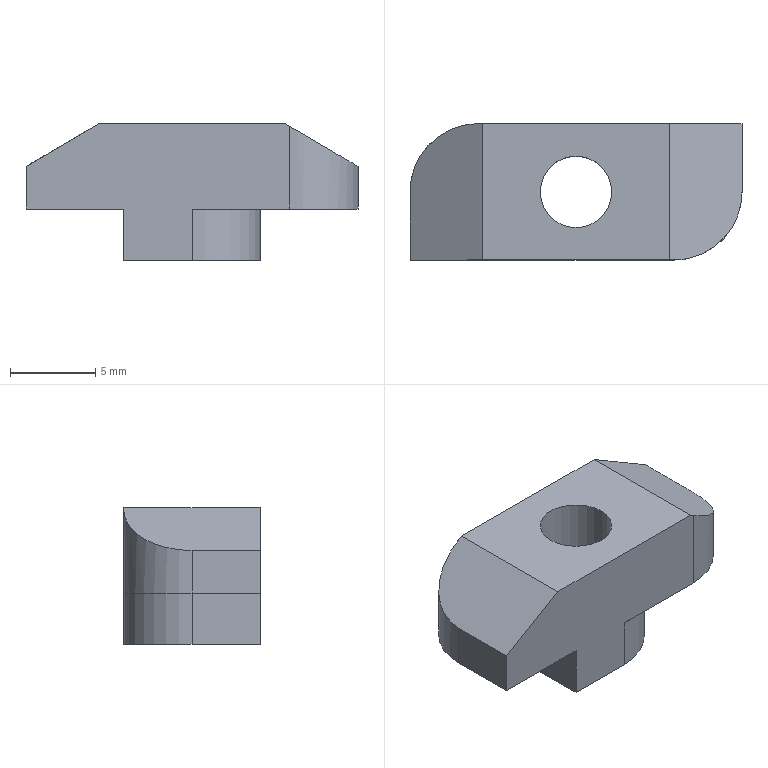Part | NX | features BREP 1 | 1 solid | 18 faces | box 19.5 x 8 x 8 mm | volume 734.785 mm3 | plane 12 | cylinder 6 | commonest cylinder face diameters 8 x4 4.2 x2
STEP:
#1=CARTESIAN_POINT('',(-2.1,0.,-8.));
#2=VERTEX_POINT('',#1);
#3=CARTESIAN_POINT('',(2.1,0.,-8.));
#4=VERTEX_POINT('',#3);
#5=CARTESIAN_POINT('',(0.,0.,-8.));
#6=DIRECTION('',(0.,0.,-1.));
#7=DIRECTION('',(-1.,0.,0.));
#8=AXIS2_PLACEMENT_3D('',#5,#6,#7);
#9=CIRCLE('',#8,2.1);
#10=EDGE_CURVE('',#2,#4,#9,.T.);
#11=ORIENTED_EDGE('',*,*,#10,.T.);
#12=CARTESIAN_POINT('',(2.1,0.,0.));
#13=VERTEX_POINT('',#12);
#14=CARTESIAN_POINT('',(2.1,0.,0.));
#15=DIRECTION('',(0.,0.,1.));
#16=VECTOR('',#15,1000.);
#17=LINE('',#14,#16);
#18=EDGE_CURVE('',#4,#13,#17,.T.);
#19=ORIENTED_EDGE('',*,*,#18,.T.);
#20=CARTESIAN_POINT('',(-2.1,0.,0.));
#21=VERTEX_POINT('',#20);
#22=CARTESIAN_POINT('',(0.,0.,0.));
#23=DIRECTION('',(0.,0.,-1.));
#24=DIRECTION('',(-1.,0.,0.));
#25=AXIS2_PLACEMENT_3D('',#22,#23,#24);
#26=CIRCLE('',#25,2.1);
#27=EDGE_CURVE('',#21,#13,#26,.T.);
#28=ORIENTED_EDGE('',*,*,#27,.F.);
#29=CARTESIAN_POINT('',(-2.1,0.,0.));
#30=DIRECTION('',(0.,0.,1.));
#31=VECTOR('',#30,1000.);
#32=LINE('',#29,#31);
#33=EDGE_CURVE('',#2,#21,#32,.T.);
#34=ORIENTED_EDGE('',*,*,#33,.F.);
#35=EDGE_LOOP('',(#11,#19,#28,#34));
#36=FACE_BOUND('',#35,.T.);
#37=CARTESIAN_POINT('',(0.,0.,0.));
#38=DIRECTION('',(0.,0.,1.));
#39=DIRECTION('',(-1.,0.,0.));
#40=AXIS2_PLACEMENT_3D('',#37,#38,#39);
#41=CYLINDRICAL_SURFACE('',#40,2.1);
#42=ADVANCED_FACE('',(#36),#41,.F.);
#43=CARTESIAN_POINT('',(0.,-4.,-5.));
#44=VERTEX_POINT('',#43);
#45=CARTESIAN_POINT('',(5.75,-4.,-5.));
#46=VERTEX_POINT('',#45);
#47=CARTESIAN_POINT('',(-9.75,-4.,-5.));
#48=DIRECTION('',(1.,0.,0.));
#49=VECTOR('',#48,1000.);
#50=LINE('',#47,#49);
#51=EDGE_CURVE('',#44,#46,#50,.T.);
#52=ORIENTED_EDGE('',*,*,#51,.F.);
#53=CARTESIAN_POINT('',(4.,0.,-5.));
#54=VERTEX_POINT('',#53);
#55=CARTESIAN_POINT('',(0.,0.,-5.));
#56=DIRECTION('',(0.,0.,-1.));
#57=DIRECTION('',(1.,0.,0.));
#58=AXIS2_PLACEMENT_3D('',#55,#56,#57);
#59=CIRCLE('',#58,4.);
#60=EDGE_CURVE('',#54,#44,#59,.T.);
#61=ORIENTED_EDGE('',*,*,#60,.F.);
#62=CARTESIAN_POINT('',(4.,4.,-5.));
#63=VERTEX_POINT('',#62);
#64=CARTESIAN_POINT('',(4.,-4.,-5.));
#65=DIRECTION('',(0.,1.,0.));
#66=VECTOR('',#65,1000.);
#67=LINE('',#64,#66);
#68=EDGE_CURVE('',#54,#63,#67,.T.);
#69=ORIENTED_EDGE('',*,*,#68,.T.);
#70=CARTESIAN_POINT('',(9.75,4.,-5.));
#71=VERTEX_POINT('',#70);
#72=CARTESIAN_POINT('',(-9.75,4.,-5.));
#73=DIRECTION('',(-1.,0.,0.));
#74=VECTOR('',#73,1000.);
#75=LINE('',#72,#74);
#76=EDGE_CURVE('',#71,#63,#75,.T.);
#77=ORIENTED_EDGE('',*,*,#76,.F.);
#78=CARTESIAN_POINT('',(9.75,0.,-5.));
#79=VERTEX_POINT('',#78);
#80=CARTESIAN_POINT('',(9.75,4.,-5.));
#81=DIRECTION('',(0.,1.,0.));
#82=VECTOR('',#81,1000.);
#83=LINE('',#80,#82);
#84=EDGE_CURVE('',#79,#71,#83,.T.);
#85=ORIENTED_EDGE('',*,*,#84,.F.);
#86=CARTESIAN_POINT('',(5.75,0.,-5.));
#87=DIRECTION('',(0.,0.,1.));
#88=DIRECTION('',(1.,0.,0.));
#89=AXIS2_PLACEMENT_3D('',#86,#87,#88);
#90=CIRCLE('',#89,4.);
#91=EDGE_CURVE('',#46,#79,#90,.T.);
#92=ORIENTED_EDGE('',*,*,#91,.F.);
#93=EDGE_LOOP('',(#52,#61,#69,#77,#85,#92));
#94=FACE_BOUND('',#93,.T.);
#95=CARTESIAN_POINT('',(0.,0.,-5.));
#96=DIRECTION('',(0.,0.,-1.));
#97=DIRECTION('',(0.,-1.,0.));
#98=AXIS2_PLACEMENT_3D('',#95,#96,#97);
#99=PLANE('',#98);
#100=ADVANCED_FACE('',(#94),#99,.T.);
#101=ORIENTED_EDGE('',*,*,#84,.T.);
#102=CARTESIAN_POINT('',(9.75,4.,-2.5));
#103=VERTEX_POINT('',#102);
#104=CARTESIAN_POINT('',(9.75,4.,-5.));
#105=DIRECTION('',(0.,0.,1.));
#106=VECTOR('',#105,1000.);
#107=LINE('',#104,#106);
#108=EDGE_CURVE('',#71,#103,#107,.T.);
#109=ORIENTED_EDGE('',*,*,#108,.T.);
#110=CARTESIAN_POINT('',(9.75,0.,-2.5));
#111=VERTEX_POINT('',#110);
#112=CARTESIAN_POINT('',(9.75,4.,-2.5));
#113=DIRECTION('',(0.,1.,0.));
#114=VECTOR('',#113,1000.);
#115=LINE('',#112,#114);
#116=EDGE_CURVE('',#111,#103,#115,.T.);
#117=ORIENTED_EDGE('',*,*,#116,.F.);
#118=CARTESIAN_POINT('',(9.75,0.,-5.));
#119=DIRECTION('',(0.,0.,1.));
#120=VECTOR('',#119,1000.);
#121=LINE('',#118,#120);
#122=EDGE_CURVE('',#79,#111,#121,.T.);
#123=ORIENTED_EDGE('',*,*,#122,.F.);
#124=EDGE_LOOP('',(#101,#109,#117,#123));
#125=FACE_BOUND('',#124,.T.);
#126=CARTESIAN_POINT('',(9.75,4.,-5.));
#127=DIRECTION('',(-1.,0.,0.));
#128=DIRECTION('',(0.,0.,1.));
#129=AXIS2_PLACEMENT_3D('',#126,#127,#128);
#130=PLANE('',#129);
#131=ADVANCED_FACE('',(#125),#130,.F.);
#132=CARTESIAN_POINT('',(-5.5,4.,0.));
#133=VERTEX_POINT('',#132);
#134=CARTESIAN_POINT('',(-5.75,4.,-0.1471));
#135=VERTEX_POINT('',#134);
#136=CARTESIAN_POINT('',(-9.75,4.,-2.5));
#137=DIRECTION('',(-0.8619,0.,-0.507));
#138=VECTOR('',#137,1000.);
#139=LINE('',#136,#138);
#140=EDGE_CURVE('',#133,#135,#139,.T.);
#141=ORIENTED_EDGE('',*,*,#140,.F.);
#142=CARTESIAN_POINT('',(5.5,4.,0.));
#143=VERTEX_POINT('',#142);
#144=CARTESIAN_POINT('',(-9.75,4.,0.));
#145=DIRECTION('',(-1.,0.,0.));
#146=VECTOR('',#145,1000.);
#147=LINE('',#144,#146);
#148=EDGE_CURVE('',#143,#133,#147,.T.);
#149=ORIENTED_EDGE('',*,*,#148,.F.);
#150=CARTESIAN_POINT('',(9.75,4.,-2.5));
#151=DIRECTION('',(-0.8619,0.,0.507));
#152=VECTOR('',#151,1000.);
#153=LINE('',#150,#152);
#154=EDGE_CURVE('',#103,#143,#153,.T.);
#155=ORIENTED_EDGE('',*,*,#154,.F.);
#156=ORIENTED_EDGE('',*,*,#108,.F.);
#157=ORIENTED_EDGE('',*,*,#76,.T.);
#158=CARTESIAN_POINT('',(4.,4.,-8.));
#159=VERTEX_POINT('',#158);
#160=CARTESIAN_POINT('',(4.,4.,-8.));
#161=DIRECTION('',(0.,0.,1.));
#162=VECTOR('',#161,1000.);
#163=LINE('',#160,#162);
#164=EDGE_CURVE('',#159,#63,#163,.T.);
#165=ORIENTED_EDGE('',*,*,#164,.F.);
#166=CARTESIAN_POINT('',(0.,4.,-8.));
#167=VERTEX_POINT('',#166);
#168=CARTESIAN_POINT('',(-4.,4.,-8.));
#169=DIRECTION('',(-1.,0.,0.));
#170=VECTOR('',#169,1000.);
#171=LINE('',#168,#170);
#172=EDGE_CURVE('',#159,#167,#171,.T.);
#173=ORIENTED_EDGE('',*,*,#172,.T.);
#174=CARTESIAN_POINT('',(0.,4.,-5.));
#175=VERTEX_POINT('',#174);
#176=CARTESIAN_POINT('',(0.,4.,-5.));
#177=DIRECTION('',(0.,0.,-1.));
#178=VECTOR('',#177,1000.);
#179=LINE('',#176,#178);
#180=EDGE_CURVE('',#175,#167,#179,.T.);
#181=ORIENTED_EDGE('',*,*,#180,.F.);
#182=CARTESIAN_POINT('',(-5.75,4.,-5.));
#183=VERTEX_POINT('',#182);
#184=CARTESIAN_POINT('',(-9.75,4.,-5.));
#185=DIRECTION('',(-1.,0.,0.));
#186=VECTOR('',#185,1000.);
#187=LINE('',#184,#186);
#188=EDGE_CURVE('',#175,#183,#187,.T.);
#189=ORIENTED_EDGE('',*,*,#188,.T.);
#190=CARTESIAN_POINT('',(-5.75,4.,-5.));
#191=DIRECTION('',(0.,0.,-1.));
#192=VECTOR('',#191,1000.);
#193=LINE('',#190,#192);
#194=EDGE_CURVE('',#135,#183,#193,.T.);
#195=ORIENTED_EDGE('',*,*,#194,.F.);
#196=EDGE_LOOP('',(#141,#149,#155,#156,#157,#165,#173,#181,#189,#195));
#197=FACE_BOUND('',#196,.T.);
#198=CARTESIAN_POINT('',(-9.75,4.,-5.));
#199=DIRECTION('',(0.,-1.,0.));
#200=DIRECTION('',(0.,0.,-1.));
#201=AXIS2_PLACEMENT_3D('',#198,#199,#200);
#202=PLANE('',#201);
#203=ADVANCED_FACE('',(#197),#202,.F.);
#204=CARTESIAN_POINT('',(-9.75,0.,-5.));
#205=VERTEX_POINT('',#204);
#206=CARTESIAN_POINT('',(-9.75,-4.,-5.));
#207=VERTEX_POINT('',#206);
#208=CARTESIAN_POINT('',(-9.75,4.,-5.));
#209=DIRECTION('',(0.,-1.,0.));
#210=VECTOR('',#209,1000.);
#211=LINE('',#208,#210);
#212=EDGE_CURVE('',#205,#207,#211,.T.);
#213=ORIENTED_EDGE('',*,*,#212,.T.);
#214=CARTESIAN_POINT('',(-9.75,-4.,-2.5));
#215=VERTEX_POINT('',#214);
#216=CARTESIAN_POINT('',(-9.75,-4.,-5.));
#217=DIRECTION('',(0.,0.,1.));
#218=VECTOR('',#217,1000.);
#219=LINE('',#216,#218);
#220=EDGE_CURVE('',#207,#215,#219,.T.);
#221=ORIENTED_EDGE('',*,*,#220,.T.);
#222=CARTESIAN_POINT('',(-9.75,0.,-2.5));
#223=VERTEX_POINT('',#222);
#224=CARTESIAN_POINT('',(-9.75,4.,-2.5));
#225=DIRECTION('',(0.,-1.,0.));
#226=VECTOR('',#225,1000.);
#227=LINE('',#224,#226);
#228=EDGE_CURVE('',#223,#215,#227,.T.);
#229=ORIENTED_EDGE('',*,*,#228,.F.);
#230=CARTESIAN_POINT('',(-9.75,0.,-5.));
#231=DIRECTION('',(0.,0.,1.));
#232=VECTOR('',#231,1000.);
#233=LINE('',#230,#232);
#234=EDGE_CURVE('',#205,#223,#233,.T.);
#235=ORIENTED_EDGE('',*,*,#234,.F.);
#236=EDGE_LOOP('',(#213,#221,#229,#235));
#237=FACE_BOUND('',#236,.T.);
#238=CARTESIAN_POINT('',(-9.75,4.,-5.));
#239=DIRECTION('',(1.,0.,0.));
#240=DIRECTION('',(0.,1.,0.));
#241=AXIS2_PLACEMENT_3D('',#238,#239,#240);
#242=PLANE('',#241);
#243=ADVANCED_FACE('',(#237),#242,.F.);
#244=CARTESIAN_POINT('',(5.5,-4.,0.));
#245=VERTEX_POINT('',#244);
#246=CARTESIAN_POINT('',(5.75,-4.,-0.1471));
#247=VERTEX_POINT('',#246);
#248=CARTESIAN_POINT('',(9.75,-4.,-2.5));
#249=DIRECTION('',(0.8619,0.,-0.507));
#250=VECTOR('',#249,1000.);
#251=LINE('',#248,#250);
#252=EDGE_CURVE('',#245,#247,#251,.T.);
#253=ORIENTED_EDGE('',*,*,#252,.F.);
#254=CARTESIAN_POINT('',(-5.5,-4.,0.));
#255=VERTEX_POINT('',#254);
#256=CARTESIAN_POINT('',(-9.75,-4.,0.));
#257=DIRECTION('',(1.,0.,0.));
#258=VECTOR('',#257,1000.);
#259=LINE('',#256,#258);
#260=EDGE_CURVE('',#255,#245,#259,.T.);
#261=ORIENTED_EDGE('',*,*,#260,.F.);
#262=CARTESIAN_POINT('',(-9.75,-4.,-2.5));
#263=DIRECTION('',(0.8619,0.,0.507));
#264=VECTOR('',#263,1000.);
#265=LINE('',#262,#264);
#266=EDGE_CURVE('',#215,#255,#265,.T.);
#267=ORIENTED_EDGE('',*,*,#266,.F.);
#268=ORIENTED_EDGE('',*,*,#220,.F.);
#269=CARTESIAN_POINT('',(-4.,-4.,-5.));
#270=VERTEX_POINT('',#269);
#271=CARTESIAN_POINT('',(-9.75,-4.,-5.));
#272=DIRECTION('',(1.,0.,0.));
#273=VECTOR('',#272,1000.);
#274=LINE('',#271,#273);
#275=EDGE_CURVE('',#207,#270,#274,.T.);
#276=ORIENTED_EDGE('',*,*,#275,.T.);
#277=CARTESIAN_POINT('',(-4.,-4.,-8.));
#278=VERTEX_POINT('',#277);
#279=CARTESIAN_POINT('',(-4.,-4.,-8.));
#280=DIRECTION('',(0.,0.,1.));
#281=VECTOR('',#280,1000.);
#282=LINE('',#279,#281);
#283=EDGE_CURVE('',#278,#270,#282,.T.);
#284=ORIENTED_EDGE('',*,*,#283,.F.);
#285=CARTESIAN_POINT('',(0.,-4.,-8.));
#286=VERTEX_POINT('',#285);
#287=CARTESIAN_POINT('',(-4.,-4.,-8.));
#288=DIRECTION('',(1.,0.,0.));
#289=VECTOR('',#288,1000.);
#290=LINE('',#287,#289);
#291=EDGE_CURVE('',#278,#286,#290,.T.);
#292=ORIENTED_EDGE('',*,*,#291,.T.);
#293=CARTESIAN_POINT('',(0.,-4.,-5.));
#294=DIRECTION('',(0.,0.,-1.));
#295=VECTOR('',#294,1000.);
#296=LINE('',#293,#295);
#297=EDGE_CURVE('',#44,#286,#296,.T.);
#298=ORIENTED_EDGE('',*,*,#297,.F.);
#299=ORIENTED_EDGE('',*,*,#51,.T.);
#300=CARTESIAN_POINT('',(5.75,-4.,-5.));
#301=DIRECTION('',(0.,0.,-1.));
#302=VECTOR('',#301,1000.);
#303=LINE('',#300,#302);
#304=EDGE_CURVE('',#247,#46,#303,.T.);
#305=ORIENTED_EDGE('',*,*,#304,.F.);
#306=EDGE_LOOP('',(#253,#261,#267,#268,#276,#284,#292,#298,#299,#305));
#307=FACE_BOUND('',#306,.T.);
#308=CARTESIAN_POINT('',(-9.75,-4.,-5.));
#309=DIRECTION('',(0.,1.,0.));
#310=DIRECTION('',(1.,0.,0.));
#311=AXIS2_PLACEMENT_3D('',#308,#309,#310);
#312=PLANE('',#311);
#313=ADVANCED_FACE('',(#307),#312,.F.);
#314=ORIENTED_EDGE('',*,*,#188,.F.);
#315=CARTESIAN_POINT('',(-4.,0.,-5.));
#316=VERTEX_POINT('',#315);
#317=CARTESIAN_POINT('',(0.,0.,-5.));
#318=DIRECTION('',(0.,0.,-1.));
#319=DIRECTION('',(1.,0.,0.));
#320=AXIS2_PLACEMENT_3D('',#317,#318,#319);
#321=CIRCLE('',#320,4.);
#322=EDGE_CURVE('',#316,#175,#321,.T.);
#323=ORIENTED_EDGE('',*,*,#322,.F.);
#324=CARTESIAN_POINT('',(-4.,-4.,-5.));
#325=DIRECTION('',(0.,-1.,0.));
#326=VECTOR('',#325,1000.);
#327=LINE('',#324,#326);
#328=EDGE_CURVE('',#316,#270,#327,.T.);
#329=ORIENTED_EDGE('',*,*,#328,.T.);
#330=ORIENTED_EDGE('',*,*,#275,.F.);
#331=ORIENTED_EDGE('',*,*,#212,.F.);
#332=CARTESIAN_POINT('',(-5.75,0.,-5.));
#333=DIRECTION('',(0.,0.,1.));
#334=DIRECTION('',(1.,0.,0.));
#335=AXIS2_PLACEMENT_3D('',#332,#333,#334);
#336=CIRCLE('',#335,4.);
#337=EDGE_CURVE('',#183,#205,#336,.T.);
#338=ORIENTED_EDGE('',*,*,#337,.F.);
#339=EDGE_LOOP('',(#314,#323,#329,#330,#331,#338));
#340=FACE_BOUND('',#339,.T.);
#341=CARTESIAN_POINT('',(0.,0.,-5.));
#342=DIRECTION('',(0.,0.,-1.));
#343=DIRECTION('',(0.,-1.,0.));
#344=AXIS2_PLACEMENT_3D('',#341,#342,#343);
#345=PLANE('',#344);
#346=ADVANCED_FACE('',(#340),#345,.T.);
#347=ORIENTED_EDGE('',*,*,#148,.T.);
#348=CARTESIAN_POINT('',(-5.5,0.,0.));
#349=DIRECTION('',(0.,1.,0.));
#350=VECTOR('',#349,1000.);
#351=LINE('',#348,#350);
#352=EDGE_CURVE('',#255,#133,#351,.T.);
#353=ORIENTED_EDGE('',*,*,#352,.F.);
#354=ORIENTED_EDGE('',*,*,#260,.T.);
#355=CARTESIAN_POINT('',(5.5,0.,0.));
#356=DIRECTION('',(0.,-1.,0.));
#357=VECTOR('',#356,1000.);
#358=LINE('',#355,#357);
#359=EDGE_CURVE('',#143,#245,#358,.T.);
#360=ORIENTED_EDGE('',*,*,#359,.F.);
#361=EDGE_LOOP('',(#347,#353,#354,#360));
#362=FACE_BOUND('',#361,.T.);
#363=ORIENTED_EDGE('',*,*,#27,.T.);
#364=CARTESIAN_POINT('',(0.,0.,0.));
#365=DIRECTION('',(0.,0.,-1.));
#366=DIRECTION('',(-1.,0.,0.));
#367=AXIS2_PLACEMENT_3D('',#364,#365,#366);
#368=CIRCLE('',#367,2.1);
#369=EDGE_CURVE('',#13,#21,#368,.T.);
#370=ORIENTED_EDGE('',*,*,#369,.T.);
#371=EDGE_LOOP('',(#363,#370));
#372=FACE_BOUND('',#371,.T.);
#373=CARTESIAN_POINT('',(0.,0.,0.));
#374=DIRECTION('',(0.,0.,-1.));
#375=DIRECTION('',(0.,-1.,0.));
#376=AXIS2_PLACEMENT_3D('',#373,#374,#375);
#377=PLANE('',#376);
#378=ADVANCED_FACE('',(#362,#372),#377,.F.);
#379=CARTESIAN_POINT('',(4.,0.,-8.));
#380=VERTEX_POINT('',#379);
#381=CARTESIAN_POINT('',(4.,-4.,-8.));
#382=DIRECTION('',(0.,1.,0.));
#383=VECTOR('',#382,1000.);
#384=LINE('',#381,#383);
#385=EDGE_CURVE('',#380,#159,#384,.T.);
#386=ORIENTED_EDGE('',*,*,#385,.T.);
#387=ORIENTED_EDGE('',*,*,#164,.T.);
#388=ORIENTED_EDGE('',*,*,#68,.F.);
#389=CARTESIAN_POINT('',(4.,0.,-8.));
#390=DIRECTION('',(0.,0.,1.));
#391=VECTOR('',#390,1000.);
#392=LINE('',#389,#391);
#393=EDGE_CURVE('',#380,#54,#392,.T.);
#394=ORIENTED_EDGE('',*,*,#393,.F.);
#395=EDGE_LOOP('',(#386,#387,#388,#394));
#396=FACE_BOUND('',#395,.T.);
#397=CARTESIAN_POINT('',(4.,-4.,-8.));
#398=DIRECTION('',(-1.,0.,0.));
#399=DIRECTION('',(0.,0.,1.));
#400=AXIS2_PLACEMENT_3D('',#397,#398,#399);
#401=PLANE('',#400);
#402=ADVANCED_FACE('',(#396),#401,.F.);
#403=CARTESIAN_POINT('',(-4.,0.,-8.));
#404=VERTEX_POINT('',#403);
#405=CARTESIAN_POINT('',(-4.,-4.,-8.));
#406=DIRECTION('',(0.,-1.,0.));
#407=VECTOR('',#406,1000.);
#408=LINE('',#405,#407);
#409=EDGE_CURVE('',#404,#278,#408,.T.);
#410=ORIENTED_EDGE('',*,*,#409,.T.);
#411=ORIENTED_EDGE('',*,*,#283,.T.);
#412=ORIENTED_EDGE('',*,*,#328,.F.);
#413=CARTESIAN_POINT('',(-4.,0.,-8.));
#414=DIRECTION('',(0.,0.,1.));
#415=VECTOR('',#414,1000.);
#416=LINE('',#413,#415);
#417=EDGE_CURVE('',#404,#316,#416,.T.);
#418=ORIENTED_EDGE('',*,*,#417,.F.);
#419=EDGE_LOOP('',(#410,#411,#412,#418));
#420=FACE_BOUND('',#419,.T.);
#421=CARTESIAN_POINT('',(-4.,-4.,-8.));
#422=DIRECTION('',(1.,0.,0.));
#423=DIRECTION('',(0.,1.,0.));
#424=AXIS2_PLACEMENT_3D('',#421,#422,#423);
#425=PLANE('',#424);
#426=ADVANCED_FACE('',(#420),#425,.F.);
#427=ORIENTED_EDGE('',*,*,#291,.F.);
#428=ORIENTED_EDGE('',*,*,#409,.F.);
#429=CARTESIAN_POINT('',(0.,0.,-8.));
#430=DIRECTION('',(0.,0.,1.));
#431=DIRECTION('',(-1.,0.,0.));
#432=AXIS2_PLACEMENT_3D('',#429,#430,#431);
#433=CIRCLE('',#432,4.);
#434=EDGE_CURVE('',#167,#404,#433,.T.);
#435=ORIENTED_EDGE('',*,*,#434,.F.);
#436=ORIENTED_EDGE('',*,*,#172,.F.);
#437=ORIENTED_EDGE('',*,*,#385,.F.);
#438=CARTESIAN_POINT('',(0.,0.,-8.));
#439=DIRECTION('',(0.,0.,1.));
#440=DIRECTION('',(-1.,0.,0.));
#441=AXIS2_PLACEMENT_3D('',#438,#439,#440);
#442=CIRCLE('',#441,4.);
#443=EDGE_CURVE('',#286,#380,#442,.T.);
#444=ORIENTED_EDGE('',*,*,#443,.F.);
#445=EDGE_LOOP('',(#427,#428,#435,#436,#437,#444));
#446=FACE_BOUND('',#445,.T.);
#447=ORIENTED_EDGE('',*,*,#10,.F.);
#448=CARTESIAN_POINT('',(0.,0.,-8.));
#449=DIRECTION('',(0.,0.,-1.));
#450=DIRECTION('',(-1.,0.,0.));
#451=AXIS2_PLACEMENT_3D('',#448,#449,#450);
#452=CIRCLE('',#451,2.1);
#453=EDGE_CURVE('',#4,#2,#452,.T.);
#454=ORIENTED_EDGE('',*,*,#453,.F.);
#455=EDGE_LOOP('',(#447,#454));
#456=FACE_BOUND('',#455,.T.);
#457=CARTESIAN_POINT('',(0.,0.,-8.));
#458=DIRECTION('',(0.,0.,1.));
#459=DIRECTION('',(1.,0.,0.));
#460=AXIS2_PLACEMENT_3D('',#457,#458,#459);
#461=PLANE('',#460);
#462=ADVANCED_FACE('',(#446,#456),#461,.F.);
#463=ORIENTED_EDGE('',*,*,#18,.F.);
#464=ORIENTED_EDGE('',*,*,#453,.T.);
#465=ORIENTED_EDGE('',*,*,#33,.T.);
#466=ORIENTED_EDGE('',*,*,#369,.F.);
#467=EDGE_LOOP('',(#463,#464,#465,#466));
#468=FACE_BOUND('',#467,.T.);
#469=CARTESIAN_POINT('',(0.,0.,0.));
#470=DIRECTION('',(0.,0.,1.));
#471=DIRECTION('',(-1.,0.,0.));
#472=AXIS2_PLACEMENT_3D('',#469,#470,#471);
#473=CYLINDRICAL_SURFACE('',#472,2.1);
#474=ADVANCED_FACE('',(#468),#473,.F.);
#475=ORIENTED_EDGE('',*,*,#116,.T.);
#476=ORIENTED_EDGE('',*,*,#154,.T.);
#477=ORIENTED_EDGE('',*,*,#359,.T.);
#478=ORIENTED_EDGE('',*,*,#252,.T.);
#479=CARTESIAN_POINT('',(9.75,0.,-2.5));
#480=CARTESIAN_POINT('',(9.75,-2.343,-2.5));
#481=CARTESIAN_POINT('',(8.093,-4.,-1.525));
#482=CARTESIAN_POINT('',(5.75,-4.,-0.1471));
#483=(BOUNDED_CURVE()B_SPLINE_CURVE(3,(#479,#480,#481,#482),.UNSPECIFIED.,.F.,.F.)B_SPLINE_CURVE_WITH_KNOTS((4,4),(3.142,4.712),.UNSPECIFIED.)CURVE()GEOMETRIC_REPRESENTATION_ITEM()RATIONAL_B_SPLINE_CURVE((1.,0.8047,0.8047,1.))REPRESENTATION_ITEM(''));
#484=EDGE_CURVE('',#111,#247,#483,.T.);
#485=ORIENTED_EDGE('',*,*,#484,.F.);
#486=EDGE_LOOP('',(#475,#476,#477,#478,#485));
#487=FACE_BOUND('',#486,.T.);
#488=CARTESIAN_POINT('',(9.75,4.,-2.5));
#489=DIRECTION('',(-0.507,0.,-0.8619));
#490=DIRECTION('',(-0.8619,0.,0.507));
#491=AXIS2_PLACEMENT_3D('',#488,#489,#490);
#492=PLANE('',#491);
#493=ADVANCED_FACE('',(#487),#492,.F.);
#494=ORIENTED_EDGE('',*,*,#228,.T.);
#495=ORIENTED_EDGE('',*,*,#266,.T.);
#496=ORIENTED_EDGE('',*,*,#352,.T.);
#497=ORIENTED_EDGE('',*,*,#140,.T.);
#498=CARTESIAN_POINT('',(-9.75,0.,-2.5));
#499=CARTESIAN_POINT('',(-9.75,2.343,-2.5));
#500=CARTESIAN_POINT('',(-8.093,4.,-1.525));
#501=CARTESIAN_POINT('',(-5.75,4.,-0.1471));
#502=(BOUNDED_CURVE()B_SPLINE_CURVE(3,(#498,#499,#500,#501),.UNSPECIFIED.,.F.,.F.)B_SPLINE_CURVE_WITH_KNOTS((4,4),(3.142,4.712),.UNSPECIFIED.)CURVE()GEOMETRIC_REPRESENTATION_ITEM()RATIONAL_B_SPLINE_CURVE((1.,0.8047,0.8047,1.))REPRESENTATION_ITEM(''));
#503=EDGE_CURVE('',#223,#135,#502,.T.);
#504=ORIENTED_EDGE('',*,*,#503,.F.);
#505=EDGE_LOOP('',(#494,#495,#496,#497,#504));
#506=FACE_BOUND('',#505,.T.);
#507=CARTESIAN_POINT('',(-9.75,4.,-2.5));
#508=DIRECTION('',(0.507,0.,-0.8619));
#509=DIRECTION('',(0.,-1.,0.));
#510=AXIS2_PLACEMENT_3D('',#507,#508,#509);
#511=PLANE('',#510);
#512=ADVANCED_FACE('',(#506),#511,.F.);
#513=ORIENTED_EDGE('',*,*,#91,.T.);
#514=ORIENTED_EDGE('',*,*,#122,.T.);
#515=ORIENTED_EDGE('',*,*,#484,.T.);
#516=ORIENTED_EDGE('',*,*,#304,.T.);
#517=EDGE_LOOP('',(#513,#514,#515,#516));
#518=FACE_BOUND('',#517,.T.);
#519=CARTESIAN_POINT('',(5.75,0.,-5.));
#520=DIRECTION('',(0.,0.,1.));
#521=DIRECTION('',(-1.,0.,0.));
#522=AXIS2_PLACEMENT_3D('',#519,#520,#521);
#523=CYLINDRICAL_SURFACE('',#522,4.);
#524=ADVANCED_FACE('',(#518),#523,.T.);
#525=ORIENTED_EDGE('',*,*,#337,.T.);
#526=ORIENTED_EDGE('',*,*,#234,.T.);
#527=ORIENTED_EDGE('',*,*,#503,.T.);
#528=ORIENTED_EDGE('',*,*,#194,.T.);
#529=EDGE_LOOP('',(#525,#526,#527,#528));
#530=FACE_BOUND('',#529,.T.);
#531=CARTESIAN_POINT('',(-5.75,0.,-5.));
#532=DIRECTION('',(0.,0.,1.));
#533=DIRECTION('',(-1.,0.,0.));
#534=AXIS2_PLACEMENT_3D('',#531,#532,#533);
#535=CYLINDRICAL_SURFACE('',#534,4.);
#536=ADVANCED_FACE('',(#530),#535,.T.);
#537=ORIENTED_EDGE('',*,*,#443,.T.);
#538=ORIENTED_EDGE('',*,*,#393,.T.);
#539=ORIENTED_EDGE('',*,*,#60,.T.);
#540=ORIENTED_EDGE('',*,*,#297,.T.);
#541=EDGE_LOOP('',(#537,#538,#539,#540));
#542=FACE_BOUND('',#541,.T.);
#543=CARTESIAN_POINT('',(0.,0.,-8.));
#544=DIRECTION('',(0.,0.,1.));
#545=DIRECTION('',(-1.,0.,0.));
#546=AXIS2_PLACEMENT_3D('',#543,#544,#545);
#547=CYLINDRICAL_SURFACE('',#546,4.);
#548=ADVANCED_FACE('',(#542),#547,.T.);
#549=ORIENTED_EDGE('',*,*,#434,.T.);
#550=ORIENTED_EDGE('',*,*,#417,.T.);
#551=ORIENTED_EDGE('',*,*,#322,.T.);
#552=ORIENTED_EDGE('',*,*,#180,.T.);
#553=EDGE_LOOP('',(#549,#550,#551,#552));
#554=FACE_BOUND('',#553,.T.);
#555=CARTESIAN_POINT('',(0.,0.,-8.));
#556=DIRECTION('',(0.,0.,1.));
#557=DIRECTION('',(-1.,0.,0.));
#558=AXIS2_PLACEMENT_3D('',#555,#556,#557);
#559=CYLINDRICAL_SURFACE('',#558,4.);
#560=ADVANCED_FACE('',(#554),#559,.T.);
#561=CLOSED_SHELL('',(#42,#100,#131,#203,#243,#313,#346,#378,#402,#426,#462,#474,#493,#512,#524,#536,#548,#560));
#562=MANIFOLD_SOLID_BREP('',#561);
#563=(LENGTH_UNIT()NAMED_UNIT(*)SI_UNIT(.MILLI.,.METRE.));
#564=UNCERTAINTY_MEASURE_WITH_UNIT(LENGTH_MEASURE(0.00001),#563,'','');
#565=(NAMED_UNIT(*)PLANE_ANGLE_UNIT()SI_UNIT($,.RADIAN.));
#566=(NAMED_UNIT(*)SI_UNIT($,.STERADIAN.)SOLID_ANGLE_UNIT());
#567=(GEOMETRIC_REPRESENTATION_CONTEXT(3)GLOBAL_UNCERTAINTY_ASSIGNED_CONTEXT((#564))GLOBAL_UNIT_ASSIGNED_CONTEXT((#563,#565,#566))REPRESENTATION_CONTEXT('',''));
#568=ADVANCED_BREP_SHAPE_REPRESENTATION('',(#562),#567);